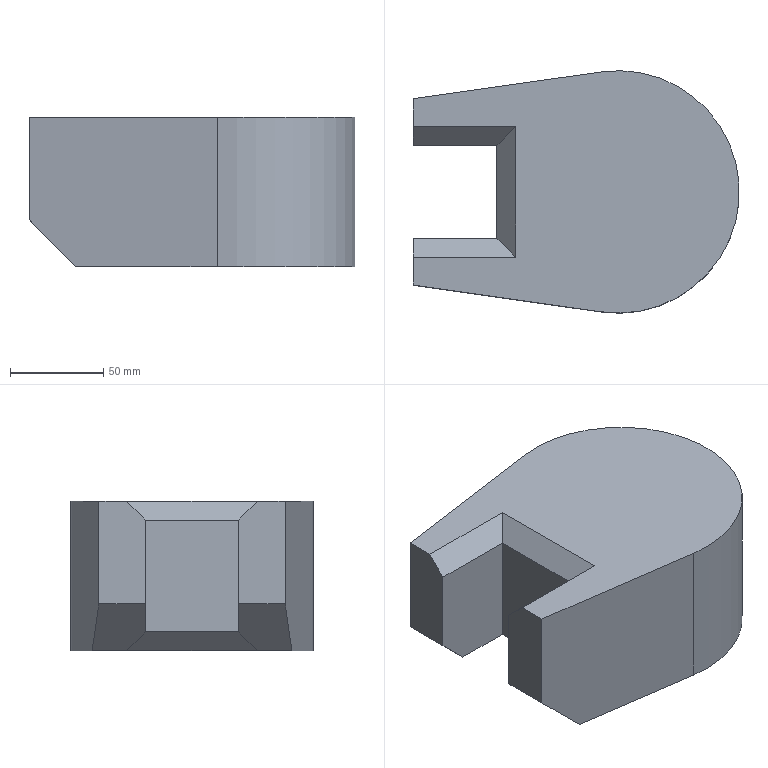Part | SolidWorks | features Chamfer 3, Extrusion 1 | 1 solid | 18 faces | box 175 x 130 x 80 mm | volume 1338839 mm3 | plane 17 | cylinder 1 | commonest cylinder face diameters 130 x1
STEP:
#1=CARTESIAN_POINT('',(-9.158,64.352,-40.));
#2=VERTEX_POINT('',#1);
#3=CARTESIAN_POINT('',(-85.,53.558,-40.));
#4=VERTEX_POINT('',#3);
#5=CARTESIAN_POINT('',(-110.,50.,-40.));
#6=DIRECTION('',(-0.99,-0.1409,0.));
#7=VECTOR('',#6,1000.);
#8=LINE('',#5,#7);
#9=EDGE_CURVE('',#2,#4,#8,.T.);
#10=ORIENTED_EDGE('',*,*,#9,.T.);
#11=CARTESIAN_POINT('',(-110.,50.,-15.));
#12=VERTEX_POINT('',#11);
#13=CARTESIAN_POINT('',(-110.,50.,-15.));
#14=DIRECTION('',(-0.7036,-0.1001,0.7036));
#15=VECTOR('',#14,1000.);
#16=LINE('',#13,#15);
#17=EDGE_CURVE('',#4,#12,#16,.T.);
#18=ORIENTED_EDGE('',*,*,#17,.T.);
#19=CARTESIAN_POINT('',(-110.,50.,40.));
#20=VERTEX_POINT('',#19);
#21=CARTESIAN_POINT('',(-110.,50.,40.));
#22=DIRECTION('',(0.,0.,-1.));
#23=VECTOR('',#22,1000.);
#24=LINE('',#21,#23);
#25=EDGE_CURVE('',#20,#12,#24,.T.);
#26=ORIENTED_EDGE('',*,*,#25,.F.);
#27=CARTESIAN_POINT('',(-9.158,64.352,40.));
#28=VERTEX_POINT('',#27);
#29=CARTESIAN_POINT('',(-110.,50.,40.));
#30=DIRECTION('',(-0.99,-0.1409,0.));
#31=VECTOR('',#30,1000.);
#32=LINE('',#29,#31);
#33=EDGE_CURVE('',#28,#20,#32,.T.);
#34=ORIENTED_EDGE('',*,*,#33,.F.);
#35=CARTESIAN_POINT('',(-9.158,64.352,40.));
#36=DIRECTION('',(0.,0.,-1.));
#37=VECTOR('',#36,1000.);
#38=LINE('',#35,#37);
#39=EDGE_CURVE('',#28,#2,#38,.T.);
#40=ORIENTED_EDGE('',*,*,#39,.T.);
#41=EDGE_LOOP('',(#10,#18,#26,#34,#40));
#42=FACE_OUTER_BOUND('',#41,.T.);
#43=CARTESIAN_POINT('',(-110.,50.,40.));
#44=DIRECTION('',(0.1409,-0.99,0.));
#45=DIRECTION('',(0.99,0.1409,0.));
#46=AXIS2_PLACEMENT_3D('',#43,#44,#45);
#47=PLANE('',#46);
#48=ADVANCED_FACE('',(#42),#47,.F.);
#49=CARTESIAN_POINT('',(-110.,25.,30.));
#50=VERTEX_POINT('',#49);
#51=CARTESIAN_POINT('',(-110.,25.,-15.));
#52=VERTEX_POINT('',#51);
#53=CARTESIAN_POINT('',(-110.,25.,40.));
#54=DIRECTION('',(0.,0.,-1.));
#55=VECTOR('',#54,1000.);
#56=LINE('',#53,#55);
#57=EDGE_CURVE('',#50,#52,#56,.T.);
#58=ORIENTED_EDGE('',*,*,#57,.F.);
#59=CARTESIAN_POINT('',(-110.,35.,40.));
#60=VERTEX_POINT('',#59);
#61=CARTESIAN_POINT('',(-110.,35.,40.));
#62=DIRECTION('',(0.,0.7071,0.7071));
#63=VECTOR('',#62,1000.);
#64=LINE('',#61,#63);
#65=EDGE_CURVE('',#50,#60,#64,.T.);
#66=ORIENTED_EDGE('',*,*,#65,.T.);
#67=CARTESIAN_POINT('',(-110.,50.,40.));
#68=DIRECTION('',(0.,-1.,0.));
#69=VECTOR('',#68,1000.);
#70=LINE('',#67,#69);
#71=EDGE_CURVE('',#20,#60,#70,.T.);
#72=ORIENTED_EDGE('',*,*,#71,.F.);
#73=ORIENTED_EDGE('',*,*,#25,.T.);
#74=CARTESIAN_POINT('',(-110.,50.,-15.));
#75=DIRECTION('',(0.,-1.,0.));
#76=VECTOR('',#75,1000.);
#77=LINE('',#74,#76);
#78=EDGE_CURVE('',#12,#52,#77,.T.);
#79=ORIENTED_EDGE('',*,*,#78,.T.);
#80=EDGE_LOOP('',(#58,#66,#72,#73,#79));
#81=FACE_OUTER_BOUND('',#80,.T.);
#82=CARTESIAN_POINT('',(-110.,50.,40.));
#83=DIRECTION('',(1.,0.,0.));
#84=DIRECTION('',(0.,0.,-1.));
#85=AXIS2_PLACEMENT_3D('',#82,#83,#84);
#86=PLANE('',#85);
#87=ADVANCED_FACE('',(#81),#86,.F.);
#88=CARTESIAN_POINT('',(-95.,25.,-30.));
#89=VERTEX_POINT('',#88);
#90=CARTESIAN_POINT('',(-110.,25.,-15.));
#91=DIRECTION('',(0.7071,0.,-0.7071));
#92=VECTOR('',#91,1000.);
#93=LINE('',#90,#92);
#94=EDGE_CURVE('',#52,#89,#93,.T.);
#95=ORIENTED_EDGE('',*,*,#94,.T.);
#96=CARTESIAN_POINT('',(-65.,25.,-30.));
#97=VERTEX_POINT('',#96);
#98=CARTESIAN_POINT('',(-110.,25.,-30.));
#99=DIRECTION('',(1.,0.,0.));
#100=VECTOR('',#99,1000.);
#101=LINE('',#98,#100);
#102=EDGE_CURVE('',#89,#97,#101,.T.);
#103=ORIENTED_EDGE('',*,*,#102,.T.);
#104=CARTESIAN_POINT('',(-65.,25.,30.));
#105=VERTEX_POINT('',#104);
#106=CARTESIAN_POINT('',(-65.,25.,40.));
#107=DIRECTION('',(0.,0.,-1.));
#108=VECTOR('',#107,1000.);
#109=LINE('',#106,#108);
#110=EDGE_CURVE('',#105,#97,#109,.T.);
#111=ORIENTED_EDGE('',*,*,#110,.F.);
#112=CARTESIAN_POINT('',(-110.,25.,30.));
#113=DIRECTION('',(-1.,0.,0.));
#114=VECTOR('',#113,1000.);
#115=LINE('',#112,#114);
#116=EDGE_CURVE('',#105,#50,#115,.T.);
#117=ORIENTED_EDGE('',*,*,#116,.T.);
#118=ORIENTED_EDGE('',*,*,#57,.T.);
#119=EDGE_LOOP('',(#95,#103,#111,#117,#118));
#120=FACE_OUTER_BOUND('',#119,.T.);
#121=CARTESIAN_POINT('',(-110.,25.,40.));
#122=DIRECTION('',(0.,1.,0.));
#123=DIRECTION('',(-1.,0.,0.));
#124=AXIS2_PLACEMENT_3D('',#121,#122,#123);
#125=PLANE('',#124);
#126=ADVANCED_FACE('',(#120),#125,.F.);
#127=ORIENTED_EDGE('',*,*,#110,.T.);
#128=CARTESIAN_POINT('',(-65.,-25.,-30.));
#129=VERTEX_POINT('',#128);
#130=CARTESIAN_POINT('',(-65.,25.,-30.));
#131=DIRECTION('',(0.,-1.,0.));
#132=VECTOR('',#131,1000.);
#133=LINE('',#130,#132);
#134=EDGE_CURVE('',#97,#129,#133,.T.);
#135=ORIENTED_EDGE('',*,*,#134,.T.);
#136=CARTESIAN_POINT('',(-65.,-25.,30.));
#137=VERTEX_POINT('',#136);
#138=CARTESIAN_POINT('',(-65.,-25.,40.));
#139=DIRECTION('',(0.,0.,-1.));
#140=VECTOR('',#139,1000.);
#141=LINE('',#138,#140);
#142=EDGE_CURVE('',#137,#129,#141,.T.);
#143=ORIENTED_EDGE('',*,*,#142,.F.);
#144=CARTESIAN_POINT('',(-65.,25.,30.));
#145=DIRECTION('',(0.,1.,0.));
#146=VECTOR('',#145,1000.);
#147=LINE('',#144,#146);
#148=EDGE_CURVE('',#137,#105,#147,.T.);
#149=ORIENTED_EDGE('',*,*,#148,.T.);
#150=EDGE_LOOP('',(#127,#135,#143,#149));
#151=FACE_OUTER_BOUND('',#150,.T.);
#152=CARTESIAN_POINT('',(-65.,25.,40.));
#153=DIRECTION('',(1.,0.,0.));
#154=DIRECTION('',(0.,0.,-1.));
#155=AXIS2_PLACEMENT_3D('',#152,#153,#154);
#156=PLANE('',#155);
#157=ADVANCED_FACE('',(#151),#156,.F.);
#158=ORIENTED_EDGE('',*,*,#142,.T.);
#159=CARTESIAN_POINT('',(-95.,-25.,-30.));
#160=VERTEX_POINT('',#159);
#161=CARTESIAN_POINT('',(-65.,-25.,-30.));
#162=DIRECTION('',(-1.,0.,0.));
#163=VECTOR('',#162,1000.);
#164=LINE('',#161,#163);
#165=EDGE_CURVE('',#129,#160,#164,.T.);
#166=ORIENTED_EDGE('',*,*,#165,.T.);
#167=CARTESIAN_POINT('',(-110.,-25.,-15.));
#168=VERTEX_POINT('',#167);
#169=CARTESIAN_POINT('',(-110.,-25.,-15.));
#170=DIRECTION('',(-0.7071,0.,0.7071));
#171=VECTOR('',#170,1000.);
#172=LINE('',#169,#171);
#173=EDGE_CURVE('',#160,#168,#172,.T.);
#174=ORIENTED_EDGE('',*,*,#173,.T.);
#175=CARTESIAN_POINT('',(-110.,-25.,30.));
#176=VERTEX_POINT('',#175);
#177=CARTESIAN_POINT('',(-110.,-25.,40.));
#178=DIRECTION('',(0.,0.,-1.));
#179=VECTOR('',#178,1000.);
#180=LINE('',#177,#179);
#181=EDGE_CURVE('',#176,#168,#180,.T.);
#182=ORIENTED_EDGE('',*,*,#181,.F.);
#183=CARTESIAN_POINT('',(-65.,-25.,30.));
#184=DIRECTION('',(1.,0.,0.));
#185=VECTOR('',#184,1000.);
#186=LINE('',#183,#185);
#187=EDGE_CURVE('',#176,#137,#186,.T.);
#188=ORIENTED_EDGE('',*,*,#187,.T.);
#189=EDGE_LOOP('',(#158,#166,#174,#182,#188));
#190=FACE_OUTER_BOUND('',#189,.T.);
#191=CARTESIAN_POINT('',(-65.,-25.,40.));
#192=DIRECTION('',(0.,-1.,0.));
#193=DIRECTION('',(1.,0.,0.));
#194=AXIS2_PLACEMENT_3D('',#191,#192,#193);
#195=PLANE('',#194);
#196=ADVANCED_FACE('',(#190),#195,.F.);
#197=CARTESIAN_POINT('',(-110.,-35.,40.));
#198=VERTEX_POINT('',#197);
#199=CARTESIAN_POINT('',(-110.,-50.,40.));
#200=VERTEX_POINT('',#199);
#201=CARTESIAN_POINT('',(-110.,-25.,40.));
#202=DIRECTION('',(0.,-1.,0.));
#203=VECTOR('',#202,1000.);
#204=LINE('',#201,#203);
#205=EDGE_CURVE('',#198,#200,#204,.T.);
#206=ORIENTED_EDGE('',*,*,#205,.F.);
#207=CARTESIAN_POINT('',(-110.,-35.,40.));
#208=DIRECTION('',(0.,0.7071,-0.7071));
#209=VECTOR('',#208,1000.);
#210=LINE('',#207,#209);
#211=EDGE_CURVE('',#198,#176,#210,.T.);
#212=ORIENTED_EDGE('',*,*,#211,.T.);
#213=ORIENTED_EDGE('',*,*,#181,.T.);
#214=CARTESIAN_POINT('',(-110.,-50.,-15.));
#215=VERTEX_POINT('',#214);
#216=CARTESIAN_POINT('',(-110.,-25.,-15.));
#217=DIRECTION('',(0.,-1.,0.));
#218=VECTOR('',#217,1000.);
#219=LINE('',#216,#218);
#220=EDGE_CURVE('',#168,#215,#219,.T.);
#221=ORIENTED_EDGE('',*,*,#220,.T.);
#222=CARTESIAN_POINT('',(-110.,-50.,40.));
#223=DIRECTION('',(0.,0.,-1.));
#224=VECTOR('',#223,1000.);
#225=LINE('',#222,#224);
#226=EDGE_CURVE('',#200,#215,#225,.T.);
#227=ORIENTED_EDGE('',*,*,#226,.F.);
#228=EDGE_LOOP('',(#206,#212,#213,#221,#227));
#229=FACE_OUTER_BOUND('',#228,.T.);
#230=CARTESIAN_POINT('',(-110.,-25.,40.));
#231=DIRECTION('',(1.,0.,0.));
#232=DIRECTION('',(0.,0.,-1.));
#233=AXIS2_PLACEMENT_3D('',#230,#231,#232);
#234=PLANE('',#233);
#235=ADVANCED_FACE('',(#229),#234,.F.);
#236=ORIENTED_EDGE('',*,*,#226,.T.);
#237=CARTESIAN_POINT('',(-85.,-53.558,-40.));
#238=VERTEX_POINT('',#237);
#239=CARTESIAN_POINT('',(-111.761,-49.749,-13.239));
#240=DIRECTION('',(0.7036,-0.1001,-0.7036));
#241=VECTOR('',#240,1000.);
#242=LINE('',#239,#241);
#243=EDGE_CURVE('',#215,#238,#242,.T.);
#244=ORIENTED_EDGE('',*,*,#243,.T.);
#245=CARTESIAN_POINT('',(-9.158,-64.352,-40.));
#246=VERTEX_POINT('',#245);
#247=CARTESIAN_POINT('',(-110.,-50.,-40.));
#248=DIRECTION('',(0.99,-0.1409,0.));
#249=VECTOR('',#248,1000.);
#250=LINE('',#247,#249);
#251=EDGE_CURVE('',#238,#246,#250,.T.);
#252=ORIENTED_EDGE('',*,*,#251,.T.);
#253=CARTESIAN_POINT('',(-9.158,-64.352,40.));
#254=VERTEX_POINT('',#253);
#255=CARTESIAN_POINT('',(-9.158,-64.352,40.));
#256=DIRECTION('',(0.,0.,-1.));
#257=VECTOR('',#256,1000.);
#258=LINE('',#255,#257);
#259=EDGE_CURVE('',#254,#246,#258,.T.);
#260=ORIENTED_EDGE('',*,*,#259,.F.);
#261=CARTESIAN_POINT('',(-110.,-50.,40.));
#262=DIRECTION('',(0.99,-0.1409,0.));
#263=VECTOR('',#262,1000.);
#264=LINE('',#261,#263);
#265=EDGE_CURVE('',#200,#254,#264,.T.);
#266=ORIENTED_EDGE('',*,*,#265,.F.);
#267=EDGE_LOOP('',(#236,#244,#252,#260,#266));
#268=FACE_OUTER_BOUND('',#267,.T.);
#269=CARTESIAN_POINT('',(-110.,-50.,40.));
#270=DIRECTION('',(0.1409,0.99,0.));
#271=DIRECTION('',(-0.99,0.1409,0.));
#272=AXIS2_PLACEMENT_3D('',#269,#270,#271);
#273=PLANE('',#272);
#274=ADVANCED_FACE('',(#268),#273,.F.);
#275=CARTESIAN_POINT('',(0.,0.,-40.));
#276=DIRECTION('',(0.,0.,1.));
#277=DIRECTION('',(1.,0.,0.));
#278=AXIS2_PLACEMENT_3D('',#275,#276,#277);
#279=CIRCLE('',#278,65.);
#280=EDGE_CURVE('',#246,#2,#279,.T.);
#281=ORIENTED_EDGE('',*,*,#280,.T.);
#282=ORIENTED_EDGE('',*,*,#39,.F.);
#283=CARTESIAN_POINT('',(0.,0.,40.));
#284=DIRECTION('',(0.,0.,1.));
#285=DIRECTION('',(1.,0.,0.));
#286=AXIS2_PLACEMENT_3D('',#283,#284,#285);
#287=CIRCLE('',#286,65.);
#288=EDGE_CURVE('',#254,#28,#287,.T.);
#289=ORIENTED_EDGE('',*,*,#288,.F.);
#290=ORIENTED_EDGE('',*,*,#259,.T.);
#291=EDGE_LOOP('',(#281,#282,#289,#290));
#292=FACE_OUTER_BOUND('',#291,.T.);
#293=CARTESIAN_POINT('',(0.,0.,40.));
#294=DIRECTION('',(0.,0.,-1.));
#295=DIRECTION('',(-1.,0.,0.));
#296=AXIS2_PLACEMENT_3D('',#293,#294,#295);
#297=CYLINDRICAL_SURFACE('',#296,65.);
#298=ADVANCED_FACE('',(#292),#297,.T.);
#299=CARTESIAN_POINT('',(-55.,35.,40.));
#300=VERTEX_POINT('',#299);
#301=CARTESIAN_POINT('',(-55.,-35.,40.));
#302=VERTEX_POINT('',#301);
#303=CARTESIAN_POINT('',(-55.,-25.,40.));
#304=DIRECTION('',(0.,-1.,0.));
#305=VECTOR('',#304,1000.);
#306=LINE('',#303,#305);
#307=EDGE_CURVE('',#300,#302,#306,.T.);
#308=ORIENTED_EDGE('',*,*,#307,.T.);
#309=CARTESIAN_POINT('',(-110.,-35.,40.));
#310=DIRECTION('',(-1.,0.,0.));
#311=VECTOR('',#310,1000.);
#312=LINE('',#309,#311);
#313=EDGE_CURVE('',#302,#198,#312,.T.);
#314=ORIENTED_EDGE('',*,*,#313,.T.);
#315=ORIENTED_EDGE('',*,*,#205,.T.);
#316=ORIENTED_EDGE('',*,*,#265,.T.);
#317=ORIENTED_EDGE('',*,*,#288,.T.);
#318=ORIENTED_EDGE('',*,*,#33,.T.);
#319=ORIENTED_EDGE('',*,*,#71,.T.);
#320=CARTESIAN_POINT('',(-65.,35.,40.));
#321=DIRECTION('',(1.,0.,0.));
#322=VECTOR('',#321,1000.);
#323=LINE('',#320,#322);
#324=EDGE_CURVE('',#60,#300,#323,.T.);
#325=ORIENTED_EDGE('',*,*,#324,.T.);
#326=EDGE_LOOP('',(#308,#314,#315,#316,#317,#318,#319,#325));
#327=FACE_OUTER_BOUND('',#326,.T.);
#328=CARTESIAN_POINT('',(0.,0.,40.));
#329=DIRECTION('',(0.,0.,1.));
#330=DIRECTION('',(1.,0.,0.));
#331=AXIS2_PLACEMENT_3D('',#328,#329,#330);
#332=PLANE('',#331);
#333=ADVANCED_FACE('',(#327),#332,.T.);
#334=CARTESIAN_POINT('',(-85.,-35.,-40.));
#335=VERTEX_POINT('',#334);
#336=CARTESIAN_POINT('',(-85.,0.,-40.));
#337=DIRECTION('',(0.,1.,0.));
#338=VECTOR('',#337,1000.);
#339=LINE('',#336,#338);
#340=EDGE_CURVE('',#238,#335,#339,.T.);
#341=ORIENTED_EDGE('',*,*,#340,.T.);
#342=CARTESIAN_POINT('',(-55.,-35.,-40.));
#343=VERTEX_POINT('',#342);
#344=CARTESIAN_POINT('',(0.,-35.,-40.));
#345=DIRECTION('',(1.,0.,0.));
#346=VECTOR('',#345,1000.);
#347=LINE('',#344,#346);
#348=EDGE_CURVE('',#335,#343,#347,.T.);
#349=ORIENTED_EDGE('',*,*,#348,.T.);
#350=CARTESIAN_POINT('',(-55.,35.,-40.));
#351=VERTEX_POINT('',#350);
#352=CARTESIAN_POINT('',(-55.,0.,-40.));
#353=DIRECTION('',(0.,1.,0.));
#354=VECTOR('',#353,1000.);
#355=LINE('',#352,#354);
#356=EDGE_CURVE('',#343,#351,#355,.T.);
#357=ORIENTED_EDGE('',*,*,#356,.T.);
#358=CARTESIAN_POINT('',(-85.,35.,-40.));
#359=VERTEX_POINT('',#358);
#360=CARTESIAN_POINT('',(0.,35.,-40.));
#361=DIRECTION('',(-1.,0.,0.));
#362=VECTOR('',#361,1000.);
#363=LINE('',#360,#362);
#364=EDGE_CURVE('',#351,#359,#363,.T.);
#365=ORIENTED_EDGE('',*,*,#364,.T.);
#366=CARTESIAN_POINT('',(-85.,0.,-40.));
#367=DIRECTION('',(0.,1.,0.));
#368=VECTOR('',#367,1000.);
#369=LINE('',#366,#368);
#370=EDGE_CURVE('',#359,#4,#369,.T.);
#371=ORIENTED_EDGE('',*,*,#370,.T.);
#372=ORIENTED_EDGE('',*,*,#9,.F.);
#373=ORIENTED_EDGE('',*,*,#280,.F.);
#374=ORIENTED_EDGE('',*,*,#251,.F.);
#375=EDGE_LOOP('',(#341,#349,#357,#365,#371,#372,#373,#374));
#376=FACE_OUTER_BOUND('',#375,.T.);
#377=CARTESIAN_POINT('',(0.,0.,-40.));
#378=DIRECTION('',(0.,0.,1.));
#379=DIRECTION('',(1.,0.,0.));
#380=AXIS2_PLACEMENT_3D('',#377,#378,#379);
#381=PLANE('',#380);
#382=ADVANCED_FACE('',(#376),#381,.F.);
#383=ORIENTED_EDGE('',*,*,#173,.F.);
#384=CARTESIAN_POINT('',(-105.,-15.,-20.));
#385=DIRECTION('',(0.5774,-0.5774,-0.5774));
#386=VECTOR('',#385,1000.);
#387=LINE('',#384,#386);
#388=EDGE_CURVE('',#160,#335,#387,.T.);
#389=ORIENTED_EDGE('',*,*,#388,.T.);
#390=ORIENTED_EDGE('',*,*,#340,.F.);
#391=ORIENTED_EDGE('',*,*,#243,.F.);
#392=ORIENTED_EDGE('',*,*,#220,.F.);
#393=EDGE_LOOP('',(#383,#389,#390,#391,#392));
#394=FACE_OUTER_BOUND('',#393,.T.);
#395=CARTESIAN_POINT('',(-110.,-25.,-15.));
#396=DIRECTION('',(0.7071,0.,0.7071));
#397=DIRECTION('',(0.,-1.,0.));
#398=AXIS2_PLACEMENT_3D('',#395,#396,#397);
#399=PLANE('',#398);
#400=ADVANCED_FACE('',(#394),#399,.F.);
#401=ORIENTED_EDGE('',*,*,#370,.F.);
#402=CARTESIAN_POINT('',(-96.667,23.333,-28.333));
#403=DIRECTION('',(-0.5774,-0.5774,0.5774));
#404=VECTOR('',#403,1000.);
#405=LINE('',#402,#404);
#406=EDGE_CURVE('',#359,#89,#405,.T.);
#407=ORIENTED_EDGE('',*,*,#406,.T.);
#408=ORIENTED_EDGE('',*,*,#94,.F.);
#409=ORIENTED_EDGE('',*,*,#78,.F.);
#410=ORIENTED_EDGE('',*,*,#17,.F.);
#411=EDGE_LOOP('',(#401,#407,#408,#409,#410));
#412=FACE_OUTER_BOUND('',#411,.T.);
#413=CARTESIAN_POINT('',(-110.,50.,-15.));
#414=DIRECTION('',(0.7071,0.,0.7071));
#415=DIRECTION('',(0.,-1.,0.));
#416=AXIS2_PLACEMENT_3D('',#413,#414,#415);
#417=PLANE('',#416);
#418=ADVANCED_FACE('',(#412),#417,.F.);
#419=ORIENTED_EDGE('',*,*,#65,.F.);
#420=ORIENTED_EDGE('',*,*,#116,.F.);
#421=CARTESIAN_POINT('',(-66.667,23.333,28.333));
#422=DIRECTION('',(-0.5774,-0.5774,-0.5774));
#423=VECTOR('',#422,1000.);
#424=LINE('',#421,#423);
#425=EDGE_CURVE('',#300,#105,#424,.T.);
#426=ORIENTED_EDGE('',*,*,#425,.F.);
#427=ORIENTED_EDGE('',*,*,#324,.F.);
#428=EDGE_LOOP('',(#419,#420,#426,#427));
#429=FACE_OUTER_BOUND('',#428,.T.);
#430=CARTESIAN_POINT('',(0.,35.,40.));
#431=DIRECTION('',(0.,-0.7071,0.7071));
#432=DIRECTION('',(-1.,0.,0.));
#433=AXIS2_PLACEMENT_3D('',#430,#431,#432);
#434=PLANE('',#433);
#435=ADVANCED_FACE('',(#429),#434,.T.);
#436=ORIENTED_EDGE('',*,*,#425,.T.);
#437=ORIENTED_EDGE('',*,*,#148,.F.);
#438=CARTESIAN_POINT('',(-36.667,-53.333,58.333));
#439=DIRECTION('',(-0.5774,0.5774,-0.5774));
#440=VECTOR('',#439,1000.);
#441=LINE('',#438,#440);
#442=EDGE_CURVE('',#302,#137,#441,.T.);
#443=ORIENTED_EDGE('',*,*,#442,.F.);
#444=ORIENTED_EDGE('',*,*,#307,.F.);
#445=EDGE_LOOP('',(#436,#437,#443,#444));
#446=FACE_OUTER_BOUND('',#445,.T.);
#447=CARTESIAN_POINT('',(-55.,0.,40.));
#448=DIRECTION('',(-0.7071,0.,0.7071));
#449=DIRECTION('',(0.,1.,0.));
#450=AXIS2_PLACEMENT_3D('',#447,#448,#449);
#451=PLANE('',#450);
#452=ADVANCED_FACE('',(#446),#451,.T.);
#453=ORIENTED_EDGE('',*,*,#442,.T.);
#454=ORIENTED_EDGE('',*,*,#187,.F.);
#455=ORIENTED_EDGE('',*,*,#211,.F.);
#456=ORIENTED_EDGE('',*,*,#313,.F.);
#457=EDGE_LOOP('',(#453,#454,#455,#456));
#458=FACE_OUTER_BOUND('',#457,.T.);
#459=CARTESIAN_POINT('',(0.,-35.,40.));
#460=DIRECTION('',(0.,0.7071,0.7071));
#461=DIRECTION('',(1.,0.,0.));
#462=AXIS2_PLACEMENT_3D('',#459,#460,#461);
#463=PLANE('',#462);
#464=ADVANCED_FACE('',(#458),#463,.T.);
#465=ORIENTED_EDGE('',*,*,#406,.F.);
#466=ORIENTED_EDGE('',*,*,#364,.F.);
#467=CARTESIAN_POINT('',(-65.,25.,-30.));
#468=DIRECTION('',(0.5774,0.5774,-0.5774));
#469=VECTOR('',#468,1000.);
#470=LINE('',#467,#469);
#471=EDGE_CURVE('',#97,#351,#470,.T.);
#472=ORIENTED_EDGE('',*,*,#471,.F.);
#473=ORIENTED_EDGE('',*,*,#102,.F.);
#474=EDGE_LOOP('',(#465,#466,#472,#473));
#475=FACE_OUTER_BOUND('',#474,.T.);
#476=CARTESIAN_POINT('',(-110.,25.,-30.));
#477=DIRECTION('',(0.,0.7071,0.7071));
#478=DIRECTION('',(1.,0.,0.));
#479=AXIS2_PLACEMENT_3D('',#476,#477,#478);
#480=PLANE('',#479);
#481=ADVANCED_FACE('',(#475),#480,.F.);
#482=ORIENTED_EDGE('',*,*,#471,.T.);
#483=ORIENTED_EDGE('',*,*,#356,.F.);
#484=CARTESIAN_POINT('',(-65.,-25.,-30.));
#485=DIRECTION('',(0.5774,-0.5774,-0.5774));
#486=VECTOR('',#485,1000.);
#487=LINE('',#484,#486);
#488=EDGE_CURVE('',#129,#343,#487,.T.);
#489=ORIENTED_EDGE('',*,*,#488,.F.);
#490=ORIENTED_EDGE('',*,*,#134,.F.);
#491=EDGE_LOOP('',(#482,#483,#489,#490));
#492=FACE_OUTER_BOUND('',#491,.T.);
#493=CARTESIAN_POINT('',(-65.,25.,-30.));
#494=DIRECTION('',(0.7071,0.,0.7071));
#495=DIRECTION('',(0.,-1.,0.));
#496=AXIS2_PLACEMENT_3D('',#493,#494,#495);
#497=PLANE('',#496);
#498=ADVANCED_FACE('',(#492),#497,.F.);
#499=ORIENTED_EDGE('',*,*,#488,.T.);
#500=ORIENTED_EDGE('',*,*,#348,.F.);
#501=ORIENTED_EDGE('',*,*,#388,.F.);
#502=ORIENTED_EDGE('',*,*,#165,.F.);
#503=EDGE_LOOP('',(#499,#500,#501,#502));
#504=FACE_OUTER_BOUND('',#503,.T.);
#505=CARTESIAN_POINT('',(-65.,-25.,-30.));
#506=DIRECTION('',(0.,-0.7071,0.7071));
#507=DIRECTION('',(-1.,0.,0.));
#508=AXIS2_PLACEMENT_3D('',#505,#506,#507);
#509=PLANE('',#508);
#510=ADVANCED_FACE('',(#504),#509,.F.);
#511=CLOSED_SHELL('',(#48,#87,#126,#157,#196,#235,#274,#298,#333,#382,#400,#418,#435,#452,#464,#481,#498,#510));
#512=MANIFOLD_SOLID_BREP('',#511);
#513=CARTESIAN_POINT('',(0.,0.,0.));
#514=DIRECTION('',(0.,0.,1.));
#515=DIRECTION('',(1.,0.,0.));
#516=AXIS2_PLACEMENT_3D('',#513,#514,#515);
#517=(LENGTH_UNIT()NAMED_UNIT(*)SI_UNIT(.MILLI.,.METRE.));
#518=UNCERTAINTY_MEASURE_WITH_UNIT(LENGTH_MEASURE(0.00001),#517,'','');
#519=(NAMED_UNIT(*)PLANE_ANGLE_UNIT()SI_UNIT($,.RADIAN.));
#520=(NAMED_UNIT(*)SI_UNIT($,.STERADIAN.)SOLID_ANGLE_UNIT());
#521=(GEOMETRIC_REPRESENTATION_CONTEXT(3)GLOBAL_UNCERTAINTY_ASSIGNED_CONTEXT((#518))GLOBAL_UNIT_ASSIGNED_CONTEXT((#517,#519,#520))REPRESENTATION_CONTEXT('',''));
#522=ADVANCED_BREP_SHAPE_REPRESENTATION('',(#512,#516),#521);